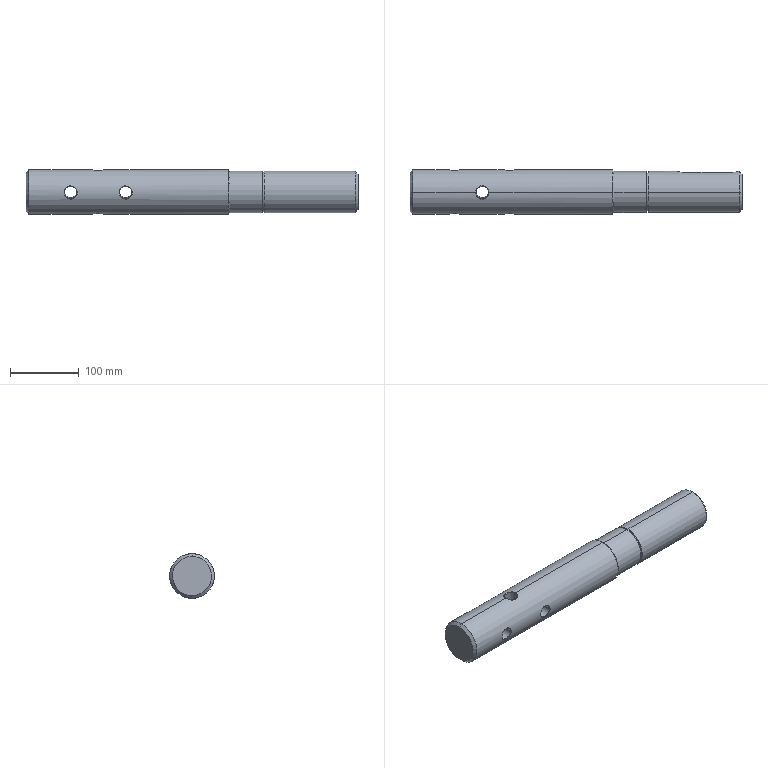Part | STEP file | Input 68 | 1 solid | 52 faces | box 483 x 65 x 65 mm | volume 1443135 mm3 | cylinder 21 | spline 12 | cone 10 | plane 9 | commonest cylinder face diameters 18 x8 60 x4 10.2 x2 12 x2 57 x2 65 x2